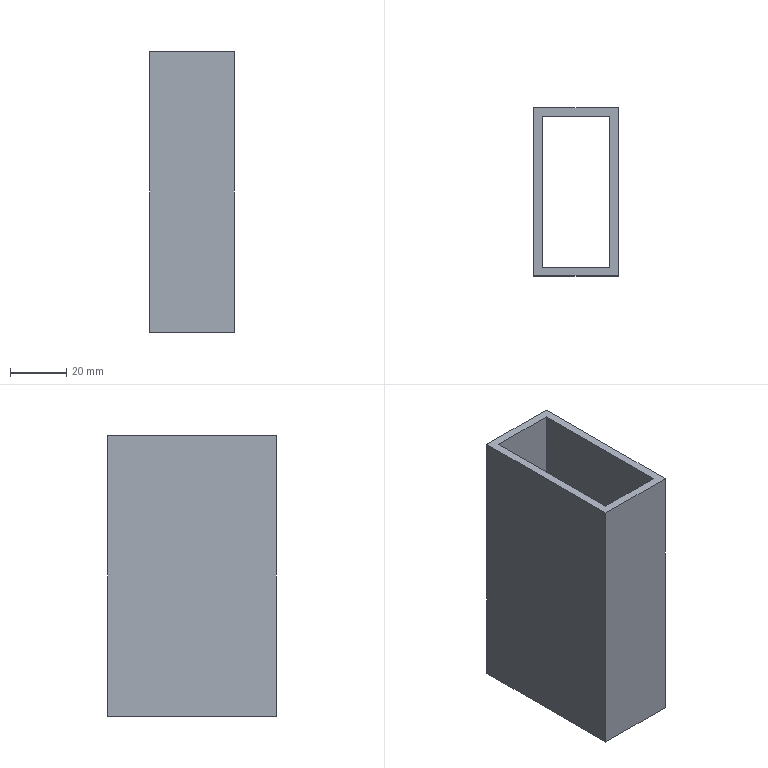Part | SolidWorks | features ExtruThin 1 | 1 solid | 10 faces | box 30 x 60 x 100 mm | volume 50400 mm3 | plane 10
STEP:
#1=CARTESIAN_POINT('',(15.,-30.,100.));
#2=VERTEX_POINT('',#1);
#3=CARTESIAN_POINT('',(15.,30.,100.));
#4=VERTEX_POINT('',#3);
#5=CARTESIAN_POINT('',(15.,-30.,100.));
#6=DIRECTION('',(0.,1.,0.));
#7=VECTOR('',#6,1000.);
#8=LINE('',#5,#7);
#9=EDGE_CURVE('',#2,#4,#8,.T.);
#10=ORIENTED_EDGE('',*,*,#9,.T.);
#11=CARTESIAN_POINT('',(-15.,30.,100.));
#12=VERTEX_POINT('',#11);
#13=CARTESIAN_POINT('',(-15.,30.,100.));
#14=DIRECTION('',(-1.,0.,0.));
#15=VECTOR('',#14,1000.);
#16=LINE('',#13,#15);
#17=EDGE_CURVE('',#4,#12,#16,.T.);
#18=ORIENTED_EDGE('',*,*,#17,.T.);
#19=CARTESIAN_POINT('',(-15.,-30.,100.));
#20=VERTEX_POINT('',#19);
#21=CARTESIAN_POINT('',(-15.,-30.,100.));
#22=DIRECTION('',(0.,-1.,0.));
#23=VECTOR('',#22,1000.);
#24=LINE('',#21,#23);
#25=EDGE_CURVE('',#12,#20,#24,.T.);
#26=ORIENTED_EDGE('',*,*,#25,.T.);
#27=CARTESIAN_POINT('',(-15.,-30.,100.));
#28=DIRECTION('',(1.,0.,0.));
#29=VECTOR('',#28,1000.);
#30=LINE('',#27,#29);
#31=EDGE_CURVE('',#20,#2,#30,.T.);
#32=ORIENTED_EDGE('',*,*,#31,.T.);
#33=EDGE_LOOP('',(#10,#18,#26,#32));
#34=FACE_OUTER_BOUND('',#33,.T.);
#35=CARTESIAN_POINT('',(12.,27.,100.));
#36=VERTEX_POINT('',#35);
#37=CARTESIAN_POINT('',(-12.,27.,100.));
#38=VERTEX_POINT('',#37);
#39=CARTESIAN_POINT('',(0.,27.,100.));
#40=DIRECTION('',(-1.,0.,0.));
#41=VECTOR('',#40,1000.);
#42=LINE('',#39,#41);
#43=EDGE_CURVE('',#36,#38,#42,.T.);
#44=ORIENTED_EDGE('',*,*,#43,.F.);
#45=CARTESIAN_POINT('',(12.,-27.,100.));
#46=VERTEX_POINT('',#45);
#47=CARTESIAN_POINT('',(12.,0.,100.));
#48=DIRECTION('',(0.,1.,0.));
#49=VECTOR('',#48,1000.);
#50=LINE('',#47,#49);
#51=EDGE_CURVE('',#46,#36,#50,.T.);
#52=ORIENTED_EDGE('',*,*,#51,.F.);
#53=CARTESIAN_POINT('',(-12.,-27.,100.));
#54=VERTEX_POINT('',#53);
#55=CARTESIAN_POINT('',(0.,-27.,100.));
#56=DIRECTION('',(1.,0.,0.));
#57=VECTOR('',#56,1000.);
#58=LINE('',#55,#57);
#59=EDGE_CURVE('',#54,#46,#58,.T.);
#60=ORIENTED_EDGE('',*,*,#59,.F.);
#61=CARTESIAN_POINT('',(-12.,0.,100.));
#62=DIRECTION('',(0.,-1.,0.));
#63=VECTOR('',#62,1000.);
#64=LINE('',#61,#63);
#65=EDGE_CURVE('',#38,#54,#64,.T.);
#66=ORIENTED_EDGE('',*,*,#65,.F.);
#67=EDGE_LOOP('',(#44,#52,#60,#66));
#68=FACE_BOUND('',#67,.T.);
#69=CARTESIAN_POINT('',(0.,0.,100.));
#70=DIRECTION('',(0.,0.,1.));
#71=DIRECTION('',(1.,0.,0.));
#72=AXIS2_PLACEMENT_3D('',#69,#70,#71);
#73=PLANE('',#72);
#74=ADVANCED_FACE('',(#34,#68),#73,.T.);
#75=CARTESIAN_POINT('',(15.,-30.,0.));
#76=VERTEX_POINT('',#75);
#77=CARTESIAN_POINT('',(15.,30.,0.));
#78=VERTEX_POINT('',#77);
#79=CARTESIAN_POINT('',(15.,-30.,0.));
#80=DIRECTION('',(0.,1.,0.));
#81=VECTOR('',#80,1000.);
#82=LINE('',#79,#81);
#83=EDGE_CURVE('',#76,#78,#82,.T.);
#84=ORIENTED_EDGE('',*,*,#83,.F.);
#85=CARTESIAN_POINT('',(-15.,-30.,0.));
#86=VERTEX_POINT('',#85);
#87=CARTESIAN_POINT('',(-15.,-30.,0.));
#88=DIRECTION('',(1.,0.,0.));
#89=VECTOR('',#88,1000.);
#90=LINE('',#87,#89);
#91=EDGE_CURVE('',#86,#76,#90,.T.);
#92=ORIENTED_EDGE('',*,*,#91,.F.);
#93=CARTESIAN_POINT('',(-15.,30.,0.));
#94=VERTEX_POINT('',#93);
#95=CARTESIAN_POINT('',(-15.,-30.,0.));
#96=DIRECTION('',(0.,-1.,0.));
#97=VECTOR('',#96,1000.);
#98=LINE('',#95,#97);
#99=EDGE_CURVE('',#94,#86,#98,.T.);
#100=ORIENTED_EDGE('',*,*,#99,.F.);
#101=CARTESIAN_POINT('',(-15.,30.,0.));
#102=DIRECTION('',(-1.,0.,0.));
#103=VECTOR('',#102,1000.);
#104=LINE('',#101,#103);
#105=EDGE_CURVE('',#78,#94,#104,.T.);
#106=ORIENTED_EDGE('',*,*,#105,.F.);
#107=EDGE_LOOP('',(#84,#92,#100,#106));
#108=FACE_OUTER_BOUND('',#107,.T.);
#109=CARTESIAN_POINT('',(12.,-27.,0.));
#110=VERTEX_POINT('',#109);
#111=CARTESIAN_POINT('',(12.,27.,0.));
#112=VERTEX_POINT('',#111);
#113=CARTESIAN_POINT('',(12.,0.,0.));
#114=DIRECTION('',(0.,1.,0.));
#115=VECTOR('',#114,1000.);
#116=LINE('',#113,#115);
#117=EDGE_CURVE('',#110,#112,#116,.T.);
#118=ORIENTED_EDGE('',*,*,#117,.T.);
#119=CARTESIAN_POINT('',(-12.,27.,0.));
#120=VERTEX_POINT('',#119);
#121=CARTESIAN_POINT('',(0.,27.,0.));
#122=DIRECTION('',(-1.,0.,0.));
#123=VECTOR('',#122,1000.);
#124=LINE('',#121,#123);
#125=EDGE_CURVE('',#112,#120,#124,.T.);
#126=ORIENTED_EDGE('',*,*,#125,.T.);
#127=CARTESIAN_POINT('',(-12.,-27.,0.));
#128=VERTEX_POINT('',#127);
#129=CARTESIAN_POINT('',(-12.,0.,0.));
#130=DIRECTION('',(0.,-1.,0.));
#131=VECTOR('',#130,1000.);
#132=LINE('',#129,#131);
#133=EDGE_CURVE('',#120,#128,#132,.T.);
#134=ORIENTED_EDGE('',*,*,#133,.T.);
#135=CARTESIAN_POINT('',(0.,-27.,0.));
#136=DIRECTION('',(1.,0.,0.));
#137=VECTOR('',#136,1000.);
#138=LINE('',#135,#137);
#139=EDGE_CURVE('',#128,#110,#138,.T.);
#140=ORIENTED_EDGE('',*,*,#139,.T.);
#141=EDGE_LOOP('',(#118,#126,#134,#140));
#142=FACE_BOUND('',#141,.T.);
#143=CARTESIAN_POINT('',(0.,0.,0.));
#144=DIRECTION('',(0.,0.,1.));
#145=DIRECTION('',(1.,0.,0.));
#146=AXIS2_PLACEMENT_3D('',#143,#144,#145);
#147=PLANE('',#146);
#148=ADVANCED_FACE('',(#108,#142),#147,.F.);
#149=ORIENTED_EDGE('',*,*,#83,.T.);
#150=CARTESIAN_POINT('',(15.,30.,100.));
#151=DIRECTION('',(0.,0.,-1.));
#152=VECTOR('',#151,1000.);
#153=LINE('',#150,#152);
#154=EDGE_CURVE('',#4,#78,#153,.T.);
#155=ORIENTED_EDGE('',*,*,#154,.F.);
#156=ORIENTED_EDGE('',*,*,#9,.F.);
#157=CARTESIAN_POINT('',(15.,-30.,100.));
#158=DIRECTION('',(0.,0.,-1.));
#159=VECTOR('',#158,1000.);
#160=LINE('',#157,#159);
#161=EDGE_CURVE('',#2,#76,#160,.T.);
#162=ORIENTED_EDGE('',*,*,#161,.T.);
#163=EDGE_LOOP('',(#149,#155,#156,#162));
#164=FACE_OUTER_BOUND('',#163,.T.);
#165=CARTESIAN_POINT('',(15.,-30.,100.));
#166=DIRECTION('',(-1.,0.,0.));
#167=DIRECTION('',(0.,0.,1.));
#168=AXIS2_PLACEMENT_3D('',#165,#166,#167);
#169=PLANE('',#168);
#170=ADVANCED_FACE('',(#164),#169,.F.);
#171=ORIENTED_EDGE('',*,*,#105,.T.);
#172=CARTESIAN_POINT('',(-15.,30.,100.));
#173=DIRECTION('',(0.,0.,-1.));
#174=VECTOR('',#173,1000.);
#175=LINE('',#172,#174);
#176=EDGE_CURVE('',#12,#94,#175,.T.);
#177=ORIENTED_EDGE('',*,*,#176,.F.);
#178=ORIENTED_EDGE('',*,*,#17,.F.);
#179=ORIENTED_EDGE('',*,*,#154,.T.);
#180=EDGE_LOOP('',(#171,#177,#178,#179));
#181=FACE_OUTER_BOUND('',#180,.T.);
#182=CARTESIAN_POINT('',(-15.,30.,100.));
#183=DIRECTION('',(0.,-1.,0.));
#184=DIRECTION('',(0.,0.,-1.));
#185=AXIS2_PLACEMENT_3D('',#182,#183,#184);
#186=PLANE('',#185);
#187=ADVANCED_FACE('',(#181),#186,.F.);
#188=ORIENTED_EDGE('',*,*,#99,.T.);
#189=CARTESIAN_POINT('',(-15.,-30.,100.));
#190=DIRECTION('',(0.,0.,-1.));
#191=VECTOR('',#190,1000.);
#192=LINE('',#189,#191);
#193=EDGE_CURVE('',#20,#86,#192,.T.);
#194=ORIENTED_EDGE('',*,*,#193,.F.);
#195=ORIENTED_EDGE('',*,*,#25,.F.);
#196=ORIENTED_EDGE('',*,*,#176,.T.);
#197=EDGE_LOOP('',(#188,#194,#195,#196));
#198=FACE_OUTER_BOUND('',#197,.T.);
#199=CARTESIAN_POINT('',(-15.,-30.,100.));
#200=DIRECTION('',(1.,0.,0.));
#201=DIRECTION('',(0.,0.,-1.));
#202=AXIS2_PLACEMENT_3D('',#199,#200,#201);
#203=PLANE('',#202);
#204=ADVANCED_FACE('',(#198),#203,.F.);
#205=ORIENTED_EDGE('',*,*,#91,.T.);
#206=ORIENTED_EDGE('',*,*,#161,.F.);
#207=ORIENTED_EDGE('',*,*,#31,.F.);
#208=ORIENTED_EDGE('',*,*,#193,.T.);
#209=EDGE_LOOP('',(#205,#206,#207,#208));
#210=FACE_OUTER_BOUND('',#209,.T.);
#211=CARTESIAN_POINT('',(-15.,-30.,100.));
#212=DIRECTION('',(0.,1.,0.));
#213=DIRECTION('',(0.,0.,1.));
#214=AXIS2_PLACEMENT_3D('',#211,#212,#213);
#215=PLANE('',#214);
#216=ADVANCED_FACE('',(#210),#215,.F.);
#217=ORIENTED_EDGE('',*,*,#117,.F.);
#218=CARTESIAN_POINT('',(12.,-27.,100.));
#219=DIRECTION('',(0.,0.,-1.));
#220=VECTOR('',#219,1000.);
#221=LINE('',#218,#220);
#222=EDGE_CURVE('',#46,#110,#221,.T.);
#223=ORIENTED_EDGE('',*,*,#222,.F.);
#224=ORIENTED_EDGE('',*,*,#51,.T.);
#225=CARTESIAN_POINT('',(12.,27.,100.));
#226=DIRECTION('',(0.,0.,-1.));
#227=VECTOR('',#226,1000.);
#228=LINE('',#225,#227);
#229=EDGE_CURVE('',#36,#112,#228,.T.);
#230=ORIENTED_EDGE('',*,*,#229,.T.);
#231=EDGE_LOOP('',(#217,#223,#224,#230));
#232=FACE_OUTER_BOUND('',#231,.T.);
#233=CARTESIAN_POINT('',(12.,0.,100.));
#234=DIRECTION('',(-1.,0.,0.));
#235=DIRECTION('',(0.,0.,1.));
#236=AXIS2_PLACEMENT_3D('',#233,#234,#235);
#237=PLANE('',#236);
#238=ADVANCED_FACE('',(#232),#237,.T.);
#239=ORIENTED_EDGE('',*,*,#125,.F.);
#240=ORIENTED_EDGE('',*,*,#229,.F.);
#241=ORIENTED_EDGE('',*,*,#43,.T.);
#242=CARTESIAN_POINT('',(-12.,27.,100.));
#243=DIRECTION('',(0.,0.,-1.));
#244=VECTOR('',#243,1000.);
#245=LINE('',#242,#244);
#246=EDGE_CURVE('',#38,#120,#245,.T.);
#247=ORIENTED_EDGE('',*,*,#246,.T.);
#248=EDGE_LOOP('',(#239,#240,#241,#247));
#249=FACE_OUTER_BOUND('',#248,.T.);
#250=CARTESIAN_POINT('',(0.,27.,100.));
#251=DIRECTION('',(0.,-1.,0.));
#252=DIRECTION('',(0.,0.,-1.));
#253=AXIS2_PLACEMENT_3D('',#250,#251,#252);
#254=PLANE('',#253);
#255=ADVANCED_FACE('',(#249),#254,.T.);
#256=ORIENTED_EDGE('',*,*,#133,.F.);
#257=ORIENTED_EDGE('',*,*,#246,.F.);
#258=ORIENTED_EDGE('',*,*,#65,.T.);
#259=CARTESIAN_POINT('',(-12.,-27.,100.));
#260=DIRECTION('',(0.,0.,-1.));
#261=VECTOR('',#260,1000.);
#262=LINE('',#259,#261);
#263=EDGE_CURVE('',#54,#128,#262,.T.);
#264=ORIENTED_EDGE('',*,*,#263,.T.);
#265=EDGE_LOOP('',(#256,#257,#258,#264));
#266=FACE_OUTER_BOUND('',#265,.T.);
#267=CARTESIAN_POINT('',(-12.,0.,100.));
#268=DIRECTION('',(1.,0.,0.));
#269=DIRECTION('',(0.,0.,-1.));
#270=AXIS2_PLACEMENT_3D('',#267,#268,#269);
#271=PLANE('',#270);
#272=ADVANCED_FACE('',(#266),#271,.T.);
#273=ORIENTED_EDGE('',*,*,#139,.F.);
#274=ORIENTED_EDGE('',*,*,#263,.F.);
#275=ORIENTED_EDGE('',*,*,#59,.T.);
#276=ORIENTED_EDGE('',*,*,#222,.T.);
#277=EDGE_LOOP('',(#273,#274,#275,#276));
#278=FACE_OUTER_BOUND('',#277,.T.);
#279=CARTESIAN_POINT('',(0.,-27.,100.));
#280=DIRECTION('',(0.,1.,0.));
#281=DIRECTION('',(0.,0.,1.));
#282=AXIS2_PLACEMENT_3D('',#279,#280,#281);
#283=PLANE('',#282);
#284=ADVANCED_FACE('',(#278),#283,.T.);
#285=CLOSED_SHELL('',(#74,#148,#170,#187,#204,#216,#238,#255,#272,#284));
#286=MANIFOLD_SOLID_BREP('',#285);
#287=CARTESIAN_POINT('',(0.,0.,0.));
#288=DIRECTION('',(0.,0.,1.));
#289=DIRECTION('',(1.,0.,0.));
#290=AXIS2_PLACEMENT_3D('',#287,#288,#289);
#291=(LENGTH_UNIT()NAMED_UNIT(*)SI_UNIT(.MILLI.,.METRE.));
#292=UNCERTAINTY_MEASURE_WITH_UNIT(LENGTH_MEASURE(0.00001),#291,'','');
#293=(NAMED_UNIT(*)PLANE_ANGLE_UNIT()SI_UNIT($,.RADIAN.));
#294=(NAMED_UNIT(*)SI_UNIT($,.STERADIAN.)SOLID_ANGLE_UNIT());
#295=(GEOMETRIC_REPRESENTATION_CONTEXT(3)GLOBAL_UNCERTAINTY_ASSIGNED_CONTEXT((#292))GLOBAL_UNIT_ASSIGNED_CONTEXT((#291,#293,#294))REPRESENTATION_CONTEXT('',''));
#296=ADVANCED_BREP_SHAPE_REPRESENTATION('',(#286,#290),#295);